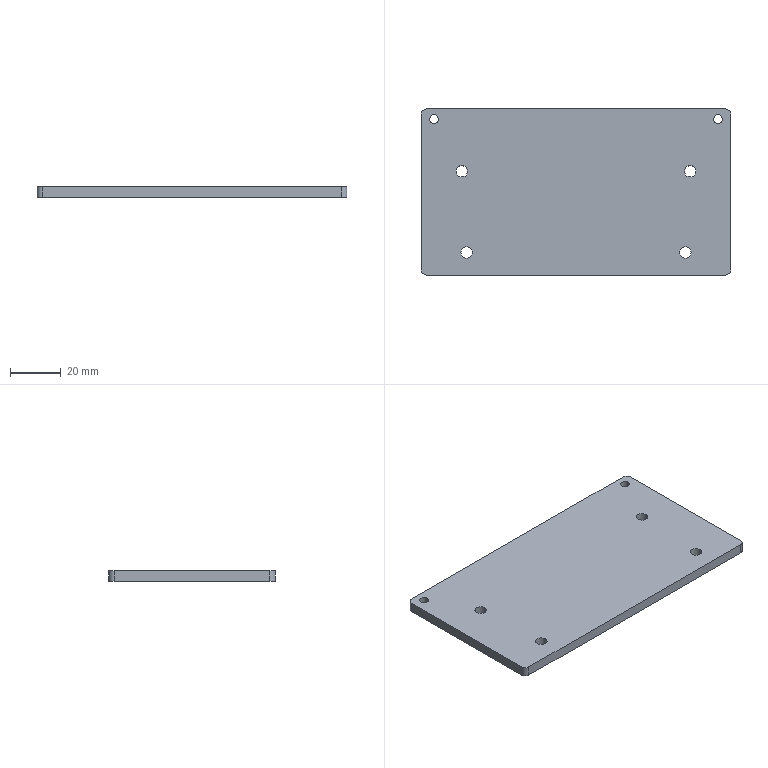Part | SolidWorks | features Extrusion 1, Fillet 1 | 1 solid | 22 faces | box 122 x 65.5 x 4 mm | volume 31619 mm3 | cylinder 16 | plane 6 | commonest cylinder face diameters 4.5 x8 3.5 x4 4 x4
STEP:
#1=CARTESIAN_POINT('',(40.9,-23.85,2.));
#2=VERTEX_POINT('',#1);
#3=CARTESIAN_POINT('',(45.4,-23.85,2.));
#4=VERTEX_POINT('',#3);
#5=CARTESIAN_POINT('',(43.15,-23.85,2.));
#6=DIRECTION('',(0.,0.,1.));
#7=DIRECTION('',(1.,0.,0.));
#8=AXIS2_PLACEMENT_3D('',#5,#6,#7);
#9=CIRCLE('',#8,2.25);
#10=EDGE_CURVE('',#2,#4,#9,.T.);
#11=ORIENTED_EDGE('',*,*,#10,.T.);
#12=CARTESIAN_POINT('',(45.4,-23.85,-2.));
#13=VERTEX_POINT('',#12);
#14=CARTESIAN_POINT('',(45.4,-23.85,2.));
#15=DIRECTION('',(0.,0.,-1.));
#16=VECTOR('',#15,1000.);
#17=LINE('',#14,#16);
#18=EDGE_CURVE('',#4,#13,#17,.T.);
#19=ORIENTED_EDGE('',*,*,#18,.T.);
#20=CARTESIAN_POINT('',(40.9,-23.85,-2.));
#21=VERTEX_POINT('',#20);
#22=CARTESIAN_POINT('',(43.15,-23.85,-2.));
#23=DIRECTION('',(0.,0.,1.));
#24=DIRECTION('',(1.,0.,0.));
#25=AXIS2_PLACEMENT_3D('',#22,#23,#24);
#26=CIRCLE('',#25,2.25);
#27=EDGE_CURVE('',#21,#13,#26,.T.);
#28=ORIENTED_EDGE('',*,*,#27,.F.);
#29=CARTESIAN_POINT('',(40.9,-23.85,2.));
#30=DIRECTION('',(0.,0.,-1.));
#31=VECTOR('',#30,1000.);
#32=LINE('',#29,#31);
#33=EDGE_CURVE('',#2,#21,#32,.T.);
#34=ORIENTED_EDGE('',*,*,#33,.F.);
#35=EDGE_LOOP('',(#11,#19,#28,#34));
#36=FACE_OUTER_BOUND('',#35,.T.);
#37=CARTESIAN_POINT('',(43.15,-23.85,2.));
#38=DIRECTION('',(0.,0.,-1.));
#39=DIRECTION('',(-1.,0.,0.));
#40=AXIS2_PLACEMENT_3D('',#37,#38,#39);
#41=CYLINDRICAL_SURFACE('',#40,2.25);
#42=ADVANCED_FACE('',(#36),#41,.F.);
#43=CARTESIAN_POINT('',(-45.4,-23.85,2.));
#44=VERTEX_POINT('',#43);
#45=CARTESIAN_POINT('',(-40.9,-23.85,2.));
#46=VERTEX_POINT('',#45);
#47=CARTESIAN_POINT('',(-43.15,-23.85,2.));
#48=DIRECTION('',(0.,0.,1.));
#49=DIRECTION('',(1.,0.,0.));
#50=AXIS2_PLACEMENT_3D('',#47,#48,#49);
#51=CIRCLE('',#50,2.25);
#52=EDGE_CURVE('',#44,#46,#51,.T.);
#53=ORIENTED_EDGE('',*,*,#52,.T.);
#54=CARTESIAN_POINT('',(-40.9,-23.85,-2.));
#55=VERTEX_POINT('',#54);
#56=CARTESIAN_POINT('',(-40.9,-23.85,2.));
#57=DIRECTION('',(0.,0.,-1.));
#58=VECTOR('',#57,1000.);
#59=LINE('',#56,#58);
#60=EDGE_CURVE('',#46,#55,#59,.T.);
#61=ORIENTED_EDGE('',*,*,#60,.T.);
#62=CARTESIAN_POINT('',(-45.4,-23.85,-2.));
#63=VERTEX_POINT('',#62);
#64=CARTESIAN_POINT('',(-43.15,-23.85,-2.));
#65=DIRECTION('',(0.,0.,1.));
#66=DIRECTION('',(1.,0.,0.));
#67=AXIS2_PLACEMENT_3D('',#64,#65,#66);
#68=CIRCLE('',#67,2.25);
#69=EDGE_CURVE('',#63,#55,#68,.T.);
#70=ORIENTED_EDGE('',*,*,#69,.F.);
#71=CARTESIAN_POINT('',(-45.4,-23.85,2.));
#72=DIRECTION('',(0.,0.,-1.));
#73=VECTOR('',#72,1000.);
#74=LINE('',#71,#73);
#75=EDGE_CURVE('',#44,#63,#74,.T.);
#76=ORIENTED_EDGE('',*,*,#75,.F.);
#77=EDGE_LOOP('',(#53,#61,#70,#76));
#78=FACE_OUTER_BOUND('',#77,.T.);
#79=CARTESIAN_POINT('',(-43.15,-23.85,2.));
#80=DIRECTION('',(0.,0.,-1.));
#81=DIRECTION('',(-1.,0.,0.));
#82=AXIS2_PLACEMENT_3D('',#79,#80,#81);
#83=CYLINDRICAL_SURFACE('',#82,2.25);
#84=ADVANCED_FACE('',(#78),#83,.F.);
#85=CARTESIAN_POINT('',(54.25,28.75,2.));
#86=VERTEX_POINT('',#85);
#87=CARTESIAN_POINT('',(57.75,28.75,2.));
#88=VERTEX_POINT('',#87);
#89=CARTESIAN_POINT('',(56.,28.75,2.));
#90=DIRECTION('',(0.,0.,1.));
#91=DIRECTION('',(-1.,0.,0.));
#92=AXIS2_PLACEMENT_3D('',#89,#90,#91);
#93=CIRCLE('',#92,1.75);
#94=EDGE_CURVE('',#86,#88,#93,.T.);
#95=ORIENTED_EDGE('',*,*,#94,.T.);
#96=CARTESIAN_POINT('',(57.75,28.75,-2.));
#97=VERTEX_POINT('',#96);
#98=CARTESIAN_POINT('',(57.75,28.75,2.));
#99=DIRECTION('',(0.,0.,-1.));
#100=VECTOR('',#99,1000.);
#101=LINE('',#98,#100);
#102=EDGE_CURVE('',#88,#97,#101,.T.);
#103=ORIENTED_EDGE('',*,*,#102,.T.);
#104=CARTESIAN_POINT('',(54.25,28.75,-2.));
#105=VERTEX_POINT('',#104);
#106=CARTESIAN_POINT('',(56.,28.75,-2.));
#107=DIRECTION('',(0.,0.,1.));
#108=DIRECTION('',(-1.,0.,0.));
#109=AXIS2_PLACEMENT_3D('',#106,#107,#108);
#110=CIRCLE('',#109,1.75);
#111=EDGE_CURVE('',#105,#97,#110,.T.);
#112=ORIENTED_EDGE('',*,*,#111,.F.);
#113=CARTESIAN_POINT('',(54.25,28.75,2.));
#114=DIRECTION('',(0.,0.,-1.));
#115=VECTOR('',#114,1000.);
#116=LINE('',#113,#115);
#117=EDGE_CURVE('',#86,#105,#116,.T.);
#118=ORIENTED_EDGE('',*,*,#117,.F.);
#119=EDGE_LOOP('',(#95,#103,#112,#118));
#120=FACE_OUTER_BOUND('',#119,.T.);
#121=CARTESIAN_POINT('',(56.,28.75,2.));
#122=DIRECTION('',(0.,0.,-1.));
#123=DIRECTION('',(-1.,0.,0.));
#124=AXIS2_PLACEMENT_3D('',#121,#122,#123);
#125=CYLINDRICAL_SURFACE('',#124,1.75);
#126=ADVANCED_FACE('',(#120),#125,.F.);
#127=CARTESIAN_POINT('',(42.75,8.15,2.));
#128=VERTEX_POINT('',#127);
#129=CARTESIAN_POINT('',(47.25,8.15,2.));
#130=VERTEX_POINT('',#129);
#131=CARTESIAN_POINT('',(45.,8.15,2.));
#132=DIRECTION('',(0.,0.,1.));
#133=DIRECTION('',(1.,0.,0.));
#134=AXIS2_PLACEMENT_3D('',#131,#132,#133);
#135=CIRCLE('',#134,2.25);
#136=EDGE_CURVE('',#128,#130,#135,.T.);
#137=ORIENTED_EDGE('',*,*,#136,.T.);
#138=CARTESIAN_POINT('',(47.25,8.15,-2.));
#139=VERTEX_POINT('',#138);
#140=CARTESIAN_POINT('',(47.25,8.15,2.));
#141=DIRECTION('',(0.,0.,-1.));
#142=VECTOR('',#141,1000.);
#143=LINE('',#140,#142);
#144=EDGE_CURVE('',#130,#139,#143,.T.);
#145=ORIENTED_EDGE('',*,*,#144,.T.);
#146=CARTESIAN_POINT('',(42.75,8.15,-2.));
#147=VERTEX_POINT('',#146);
#148=CARTESIAN_POINT('',(45.,8.15,-2.));
#149=DIRECTION('',(0.,0.,1.));
#150=DIRECTION('',(1.,0.,0.));
#151=AXIS2_PLACEMENT_3D('',#148,#149,#150);
#152=CIRCLE('',#151,2.25);
#153=EDGE_CURVE('',#147,#139,#152,.T.);
#154=ORIENTED_EDGE('',*,*,#153,.F.);
#155=CARTESIAN_POINT('',(42.75,8.15,2.));
#156=DIRECTION('',(0.,0.,-1.));
#157=VECTOR('',#156,1000.);
#158=LINE('',#155,#157);
#159=EDGE_CURVE('',#128,#147,#158,.T.);
#160=ORIENTED_EDGE('',*,*,#159,.F.);
#161=EDGE_LOOP('',(#137,#145,#154,#160));
#162=FACE_OUTER_BOUND('',#161,.T.);
#163=CARTESIAN_POINT('',(45.,8.15,2.));
#164=DIRECTION('',(0.,0.,-1.));
#165=DIRECTION('',(-1.,0.,0.));
#166=AXIS2_PLACEMENT_3D('',#163,#164,#165);
#167=CYLINDRICAL_SURFACE('',#166,2.25);
#168=ADVANCED_FACE('',(#162),#167,.F.);
#169=CARTESIAN_POINT('',(-47.25,8.15,2.));
#170=VERTEX_POINT('',#169);
#171=CARTESIAN_POINT('',(-42.75,8.15,2.));
#172=VERTEX_POINT('',#171);
#173=CARTESIAN_POINT('',(-45.,8.15,2.));
#174=DIRECTION('',(0.,0.,1.));
#175=DIRECTION('',(1.,0.,0.));
#176=AXIS2_PLACEMENT_3D('',#173,#174,#175);
#177=CIRCLE('',#176,2.25);
#178=EDGE_CURVE('',#170,#172,#177,.T.);
#179=ORIENTED_EDGE('',*,*,#178,.T.);
#180=CARTESIAN_POINT('',(-42.75,8.15,-2.));
#181=VERTEX_POINT('',#180);
#182=CARTESIAN_POINT('',(-42.75,8.15,2.));
#183=DIRECTION('',(0.,0.,-1.));
#184=VECTOR('',#183,1000.);
#185=LINE('',#182,#184);
#186=EDGE_CURVE('',#172,#181,#185,.T.);
#187=ORIENTED_EDGE('',*,*,#186,.T.);
#188=CARTESIAN_POINT('',(-47.25,8.15,-2.));
#189=VERTEX_POINT('',#188);
#190=CARTESIAN_POINT('',(-45.,8.15,-2.));
#191=DIRECTION('',(0.,0.,1.));
#192=DIRECTION('',(1.,0.,0.));
#193=AXIS2_PLACEMENT_3D('',#190,#191,#192);
#194=CIRCLE('',#193,2.25);
#195=EDGE_CURVE('',#189,#181,#194,.T.);
#196=ORIENTED_EDGE('',*,*,#195,.F.);
#197=CARTESIAN_POINT('',(-47.25,8.15,2.));
#198=DIRECTION('',(0.,0.,-1.));
#199=VECTOR('',#198,1000.);
#200=LINE('',#197,#199);
#201=EDGE_CURVE('',#170,#189,#200,.T.);
#202=ORIENTED_EDGE('',*,*,#201,.F.);
#203=EDGE_LOOP('',(#179,#187,#196,#202));
#204=FACE_OUTER_BOUND('',#203,.T.);
#205=CARTESIAN_POINT('',(-45.,8.15,2.));
#206=DIRECTION('',(0.,0.,-1.));
#207=DIRECTION('',(-1.,0.,0.));
#208=AXIS2_PLACEMENT_3D('',#205,#206,#207);
#209=CYLINDRICAL_SURFACE('',#208,2.25);
#210=ADVANCED_FACE('',(#204),#209,.F.);
#211=CARTESIAN_POINT('',(-57.75,28.75,2.));
#212=VERTEX_POINT('',#211);
#213=CARTESIAN_POINT('',(-54.25,28.75,2.));
#214=VERTEX_POINT('',#213);
#215=CARTESIAN_POINT('',(-56.,28.75,2.));
#216=DIRECTION('',(0.,0.,1.));
#217=DIRECTION('',(1.,0.,0.));
#218=AXIS2_PLACEMENT_3D('',#215,#216,#217);
#219=CIRCLE('',#218,1.75);
#220=EDGE_CURVE('',#212,#214,#219,.T.);
#221=ORIENTED_EDGE('',*,*,#220,.T.);
#222=CARTESIAN_POINT('',(-54.25,28.75,-2.));
#223=VERTEX_POINT('',#222);
#224=CARTESIAN_POINT('',(-54.25,28.75,2.));
#225=DIRECTION('',(0.,0.,-1.));
#226=VECTOR('',#225,1000.);
#227=LINE('',#224,#226);
#228=EDGE_CURVE('',#214,#223,#227,.T.);
#229=ORIENTED_EDGE('',*,*,#228,.T.);
#230=CARTESIAN_POINT('',(-57.75,28.75,-2.));
#231=VERTEX_POINT('',#230);
#232=CARTESIAN_POINT('',(-56.,28.75,-2.));
#233=DIRECTION('',(0.,0.,1.));
#234=DIRECTION('',(1.,0.,0.));
#235=AXIS2_PLACEMENT_3D('',#232,#233,#234);
#236=CIRCLE('',#235,1.75);
#237=EDGE_CURVE('',#231,#223,#236,.T.);
#238=ORIENTED_EDGE('',*,*,#237,.F.);
#239=CARTESIAN_POINT('',(-57.75,28.75,2.));
#240=DIRECTION('',(0.,0.,-1.));
#241=VECTOR('',#240,1000.);
#242=LINE('',#239,#241);
#243=EDGE_CURVE('',#212,#231,#242,.T.);
#244=ORIENTED_EDGE('',*,*,#243,.F.);
#245=EDGE_LOOP('',(#221,#229,#238,#244));
#246=FACE_OUTER_BOUND('',#245,.T.);
#247=CARTESIAN_POINT('',(-56.,28.75,2.));
#248=DIRECTION('',(0.,0.,-1.));
#249=DIRECTION('',(-1.,0.,0.));
#250=AXIS2_PLACEMENT_3D('',#247,#248,#249);
#251=CYLINDRICAL_SURFACE('',#250,1.75);
#252=ADVANCED_FACE('',(#246),#251,.F.);
#253=ORIENTED_EDGE('',*,*,#52,.F.);
#254=CARTESIAN_POINT('',(-43.15,-23.85,2.));
#255=DIRECTION('',(0.,0.,1.));
#256=DIRECTION('',(1.,0.,0.));
#257=AXIS2_PLACEMENT_3D('',#254,#255,#256);
#258=CIRCLE('',#257,2.25);
#259=EDGE_CURVE('',#46,#44,#258,.T.);
#260=ORIENTED_EDGE('',*,*,#259,.F.);
#261=EDGE_LOOP('',(#253,#260));
#262=FACE_BOUND('',#261,.T.);
#263=ORIENTED_EDGE('',*,*,#136,.F.);
#264=CARTESIAN_POINT('',(45.,8.15,2.));
#265=DIRECTION('',(0.,0.,1.));
#266=DIRECTION('',(1.,0.,0.));
#267=AXIS2_PLACEMENT_3D('',#264,#265,#266);
#268=CIRCLE('',#267,2.25);
#269=EDGE_CURVE('',#130,#128,#268,.T.);
#270=ORIENTED_EDGE('',*,*,#269,.F.);
#271=EDGE_LOOP('',(#263,#270));
#272=FACE_BOUND('',#271,.T.);
#273=ORIENTED_EDGE('',*,*,#220,.F.);
#274=CARTESIAN_POINT('',(-56.,28.75,2.));
#275=DIRECTION('',(0.,0.,1.));
#276=DIRECTION('',(1.,0.,0.));
#277=AXIS2_PLACEMENT_3D('',#274,#275,#276);
#278=CIRCLE('',#277,1.75);
#279=EDGE_CURVE('',#214,#212,#278,.T.);
#280=ORIENTED_EDGE('',*,*,#279,.F.);
#281=EDGE_LOOP('',(#273,#280));
#282=FACE_BOUND('',#281,.T.);
#283=CARTESIAN_POINT('',(-59.,-32.75,2.));
#284=VERTEX_POINT('',#283);
#285=CARTESIAN_POINT('',(59.,-32.75,2.));
#286=VERTEX_POINT('',#285);
#287=CARTESIAN_POINT('',(-61.,-32.75,2.));
#288=DIRECTION('',(1.,0.,0.));
#289=VECTOR('',#288,1000.);
#290=LINE('',#287,#289);
#291=EDGE_CURVE('',#284,#286,#290,.T.);
#292=ORIENTED_EDGE('',*,*,#291,.T.);
#293=CARTESIAN_POINT('',(61.,-30.75,2.));
#294=VERTEX_POINT('',#293);
#295=CARTESIAN_POINT('',(59.,-30.75,2.));
#296=DIRECTION('',(0.,0.,1.));
#297=DIRECTION('',(1.,0.,0.));
#298=AXIS2_PLACEMENT_3D('',#295,#296,#297);
#299=CIRCLE('',#298,2.);
#300=EDGE_CURVE('',#286,#294,#299,.T.);
#301=ORIENTED_EDGE('',*,*,#300,.T.);
#302=CARTESIAN_POINT('',(61.,30.75,2.));
#303=VERTEX_POINT('',#302);
#304=CARTESIAN_POINT('',(61.,32.75,2.));
#305=DIRECTION('',(0.,1.,0.));
#306=VECTOR('',#305,1000.);
#307=LINE('',#304,#306);
#308=EDGE_CURVE('',#294,#303,#307,.T.);
#309=ORIENTED_EDGE('',*,*,#308,.T.);
#310=CARTESIAN_POINT('',(59.,32.75,2.));
#311=VERTEX_POINT('',#310);
#312=CARTESIAN_POINT('',(59.,30.75,2.));
#313=DIRECTION('',(0.,0.,1.));
#314=DIRECTION('',(1.,0.,0.));
#315=AXIS2_PLACEMENT_3D('',#312,#313,#314);
#316=CIRCLE('',#315,2.);
#317=EDGE_CURVE('',#303,#311,#316,.T.);
#318=ORIENTED_EDGE('',*,*,#317,.T.);
#319=CARTESIAN_POINT('',(-59.,32.75,2.));
#320=VERTEX_POINT('',#319);
#321=CARTESIAN_POINT('',(-61.,32.75,2.));
#322=DIRECTION('',(-1.,0.,0.));
#323=VECTOR('',#322,1000.);
#324=LINE('',#321,#323);
#325=EDGE_CURVE('',#311,#320,#324,.T.);
#326=ORIENTED_EDGE('',*,*,#325,.T.);
#327=CARTESIAN_POINT('',(-61.,30.75,2.));
#328=VERTEX_POINT('',#327);
#329=CARTESIAN_POINT('',(-59.,30.75,2.));
#330=DIRECTION('',(0.,0.,1.));
#331=DIRECTION('',(1.,0.,0.));
#332=AXIS2_PLACEMENT_3D('',#329,#330,#331);
#333=CIRCLE('',#332,2.);
#334=EDGE_CURVE('',#320,#328,#333,.T.);
#335=ORIENTED_EDGE('',*,*,#334,.T.);
#336=CARTESIAN_POINT('',(-61.,-30.75,2.));
#337=VERTEX_POINT('',#336);
#338=CARTESIAN_POINT('',(-61.,32.75,2.));
#339=DIRECTION('',(0.,-1.,0.));
#340=VECTOR('',#339,1000.);
#341=LINE('',#338,#340);
#342=EDGE_CURVE('',#328,#337,#341,.T.);
#343=ORIENTED_EDGE('',*,*,#342,.T.);
#344=CARTESIAN_POINT('',(-59.,-30.75,2.));
#345=DIRECTION('',(0.,0.,1.));
#346=DIRECTION('',(1.,0.,0.));
#347=AXIS2_PLACEMENT_3D('',#344,#345,#346);
#348=CIRCLE('',#347,2.);
#349=EDGE_CURVE('',#337,#284,#348,.T.);
#350=ORIENTED_EDGE('',*,*,#349,.T.);
#351=EDGE_LOOP('',(#292,#301,#309,#318,#326,#335,#343,#350));
#352=FACE_OUTER_BOUND('',#351,.T.);
#353=ORIENTED_EDGE('',*,*,#178,.F.);
#354=CARTESIAN_POINT('',(-45.,8.15,2.));
#355=DIRECTION('',(0.,0.,1.));
#356=DIRECTION('',(1.,0.,0.));
#357=AXIS2_PLACEMENT_3D('',#354,#355,#356);
#358=CIRCLE('',#357,2.25);
#359=EDGE_CURVE('',#172,#170,#358,.T.);
#360=ORIENTED_EDGE('',*,*,#359,.F.);
#361=EDGE_LOOP('',(#353,#360));
#362=FACE_BOUND('',#361,.T.);
#363=ORIENTED_EDGE('',*,*,#94,.F.);
#364=CARTESIAN_POINT('',(56.,28.75,2.));
#365=DIRECTION('',(0.,0.,1.));
#366=DIRECTION('',(-1.,0.,0.));
#367=AXIS2_PLACEMENT_3D('',#364,#365,#366);
#368=CIRCLE('',#367,1.75);
#369=EDGE_CURVE('',#88,#86,#368,.T.);
#370=ORIENTED_EDGE('',*,*,#369,.F.);
#371=EDGE_LOOP('',(#363,#370));
#372=FACE_BOUND('',#371,.T.);
#373=ORIENTED_EDGE('',*,*,#10,.F.);
#374=CARTESIAN_POINT('',(43.15,-23.85,2.));
#375=DIRECTION('',(0.,0.,1.));
#376=DIRECTION('',(1.,0.,0.));
#377=AXIS2_PLACEMENT_3D('',#374,#375,#376);
#378=CIRCLE('',#377,2.25);
#379=EDGE_CURVE('',#4,#2,#378,.T.);
#380=ORIENTED_EDGE('',*,*,#379,.F.);
#381=EDGE_LOOP('',(#373,#380));
#382=FACE_BOUND('',#381,.T.);
#383=CARTESIAN_POINT('',(0.,0.,2.));
#384=DIRECTION('',(0.,0.,1.));
#385=DIRECTION('',(1.,0.,0.));
#386=AXIS2_PLACEMENT_3D('',#383,#384,#385);
#387=PLANE('',#386);
#388=ADVANCED_FACE('',(#262,#272,#282,#352,#362,#372,#382),#387,.T.);
#389=CARTESIAN_POINT('',(61.,-30.75,-2.));
#390=VERTEX_POINT('',#389);
#391=CARTESIAN_POINT('',(61.,30.75,-2.));
#392=VERTEX_POINT('',#391);
#393=CARTESIAN_POINT('',(61.,32.75,-2.));
#394=DIRECTION('',(0.,1.,0.));
#395=VECTOR('',#394,1000.);
#396=LINE('',#393,#395);
#397=EDGE_CURVE('',#390,#392,#396,.T.);
#398=ORIENTED_EDGE('',*,*,#397,.F.);
#399=CARTESIAN_POINT('',(59.,-32.75,-2.));
#400=VERTEX_POINT('',#399);
#401=CARTESIAN_POINT('',(59.,-30.75,-2.));
#402=DIRECTION('',(0.,0.,-1.));
#403=DIRECTION('',(1.,0.,0.));
#404=AXIS2_PLACEMENT_3D('',#401,#402,#403);
#405=CIRCLE('',#404,2.);
#406=EDGE_CURVE('',#390,#400,#405,.T.);
#407=ORIENTED_EDGE('',*,*,#406,.T.);
#408=CARTESIAN_POINT('',(-59.,-32.75,-2.));
#409=VERTEX_POINT('',#408);
#410=CARTESIAN_POINT('',(-61.,-32.75,-2.));
#411=DIRECTION('',(1.,0.,0.));
#412=VECTOR('',#411,1000.);
#413=LINE('',#410,#412);
#414=EDGE_CURVE('',#409,#400,#413,.T.);
#415=ORIENTED_EDGE('',*,*,#414,.F.);
#416=CARTESIAN_POINT('',(-61.,-30.75,-2.));
#417=VERTEX_POINT('',#416);
#418=CARTESIAN_POINT('',(-59.,-30.75,-2.));
#419=DIRECTION('',(0.,0.,-1.));
#420=DIRECTION('',(1.,0.,0.));
#421=AXIS2_PLACEMENT_3D('',#418,#419,#420);
#422=CIRCLE('',#421,2.);
#423=EDGE_CURVE('',#409,#417,#422,.T.);
#424=ORIENTED_EDGE('',*,*,#423,.T.);
#425=CARTESIAN_POINT('',(-61.,30.75,-2.));
#426=VERTEX_POINT('',#425);
#427=CARTESIAN_POINT('',(-61.,32.75,-2.));
#428=DIRECTION('',(0.,-1.,0.));
#429=VECTOR('',#428,1000.);
#430=LINE('',#427,#429);
#431=EDGE_CURVE('',#426,#417,#430,.T.);
#432=ORIENTED_EDGE('',*,*,#431,.F.);
#433=CARTESIAN_POINT('',(-59.,32.75,-2.));
#434=VERTEX_POINT('',#433);
#435=CARTESIAN_POINT('',(-59.,30.75,-2.));
#436=DIRECTION('',(0.,0.,-1.));
#437=DIRECTION('',(1.,0.,0.));
#438=AXIS2_PLACEMENT_3D('',#435,#436,#437);
#439=CIRCLE('',#438,2.);
#440=EDGE_CURVE('',#426,#434,#439,.T.);
#441=ORIENTED_EDGE('',*,*,#440,.T.);
#442=CARTESIAN_POINT('',(59.,32.75,-2.));
#443=VERTEX_POINT('',#442);
#444=CARTESIAN_POINT('',(-61.,32.75,-2.));
#445=DIRECTION('',(-1.,0.,0.));
#446=VECTOR('',#445,1000.);
#447=LINE('',#444,#446);
#448=EDGE_CURVE('',#443,#434,#447,.T.);
#449=ORIENTED_EDGE('',*,*,#448,.F.);
#450=CARTESIAN_POINT('',(59.,30.75,-2.));
#451=DIRECTION('',(0.,0.,-1.));
#452=DIRECTION('',(1.,0.,0.));
#453=AXIS2_PLACEMENT_3D('',#450,#451,#452);
#454=CIRCLE('',#453,2.);
#455=EDGE_CURVE('',#443,#392,#454,.T.);
#456=ORIENTED_EDGE('',*,*,#455,.T.);
#457=EDGE_LOOP('',(#398,#407,#415,#424,#432,#441,#449,#456));
#458=FACE_OUTER_BOUND('',#457,.T.);
#459=ORIENTED_EDGE('',*,*,#237,.T.);
#460=CARTESIAN_POINT('',(-56.,28.75,-2.));
#461=DIRECTION('',(0.,0.,1.));
#462=DIRECTION('',(1.,0.,0.));
#463=AXIS2_PLACEMENT_3D('',#460,#461,#462);
#464=CIRCLE('',#463,1.75);
#465=EDGE_CURVE('',#223,#231,#464,.T.);
#466=ORIENTED_EDGE('',*,*,#465,.T.);
#467=EDGE_LOOP('',(#459,#466));
#468=FACE_BOUND('',#467,.T.);
#469=ORIENTED_EDGE('',*,*,#195,.T.);
#470=CARTESIAN_POINT('',(-45.,8.15,-2.));
#471=DIRECTION('',(0.,0.,1.));
#472=DIRECTION('',(1.,0.,0.));
#473=AXIS2_PLACEMENT_3D('',#470,#471,#472);
#474=CIRCLE('',#473,2.25);
#475=EDGE_CURVE('',#181,#189,#474,.T.);
#476=ORIENTED_EDGE('',*,*,#475,.T.);
#477=EDGE_LOOP('',(#469,#476));
#478=FACE_BOUND('',#477,.T.);
#479=ORIENTED_EDGE('',*,*,#153,.T.);
#480=CARTESIAN_POINT('',(45.,8.15,-2.));
#481=DIRECTION('',(0.,0.,1.));
#482=DIRECTION('',(1.,0.,0.));
#483=AXIS2_PLACEMENT_3D('',#480,#481,#482);
#484=CIRCLE('',#483,2.25);
#485=EDGE_CURVE('',#139,#147,#484,.T.);
#486=ORIENTED_EDGE('',*,*,#485,.T.);
#487=EDGE_LOOP('',(#479,#486));
#488=FACE_BOUND('',#487,.T.);
#489=ORIENTED_EDGE('',*,*,#111,.T.);
#490=CARTESIAN_POINT('',(56.,28.75,-2.));
#491=DIRECTION('',(0.,0.,1.));
#492=DIRECTION('',(-1.,0.,0.));
#493=AXIS2_PLACEMENT_3D('',#490,#491,#492);
#494=CIRCLE('',#493,1.75);
#495=EDGE_CURVE('',#97,#105,#494,.T.);
#496=ORIENTED_EDGE('',*,*,#495,.T.);
#497=EDGE_LOOP('',(#489,#496));
#498=FACE_BOUND('',#497,.T.);
#499=ORIENTED_EDGE('',*,*,#69,.T.);
#500=CARTESIAN_POINT('',(-43.15,-23.85,-2.));
#501=DIRECTION('',(0.,0.,1.));
#502=DIRECTION('',(1.,0.,0.));
#503=AXIS2_PLACEMENT_3D('',#500,#501,#502);
#504=CIRCLE('',#503,2.25);
#505=EDGE_CURVE('',#55,#63,#504,.T.);
#506=ORIENTED_EDGE('',*,*,#505,.T.);
#507=EDGE_LOOP('',(#499,#506));
#508=FACE_BOUND('',#507,.T.);
#509=ORIENTED_EDGE('',*,*,#27,.T.);
#510=CARTESIAN_POINT('',(43.15,-23.85,-2.));
#511=DIRECTION('',(0.,0.,1.));
#512=DIRECTION('',(1.,0.,0.));
#513=AXIS2_PLACEMENT_3D('',#510,#511,#512);
#514=CIRCLE('',#513,2.25);
#515=EDGE_CURVE('',#13,#21,#514,.T.);
#516=ORIENTED_EDGE('',*,*,#515,.T.);
#517=EDGE_LOOP('',(#509,#516));
#518=FACE_BOUND('',#517,.T.);
#519=CARTESIAN_POINT('',(0.,0.,-2.));
#520=DIRECTION('',(0.,0.,1.));
#521=DIRECTION('',(1.,0.,0.));
#522=AXIS2_PLACEMENT_3D('',#519,#520,#521);
#523=PLANE('',#522);
#524=ADVANCED_FACE('',(#458,#468,#478,#488,#498,#508,#518),#523,.F.);
#525=ORIENTED_EDGE('',*,*,#308,.F.);
#526=CARTESIAN_POINT('',(61.,-30.75,2.));
#527=DIRECTION('',(0.,0.,-1.));
#528=VECTOR('',#527,1000.);
#529=LINE('',#526,#528);
#530=EDGE_CURVE('',#294,#390,#529,.T.);
#531=ORIENTED_EDGE('',*,*,#530,.T.);
#532=ORIENTED_EDGE('',*,*,#397,.T.);
#533=CARTESIAN_POINT('',(61.,30.75,2.));
#534=DIRECTION('',(0.,0.,1.));
#535=VECTOR('',#534,1000.);
#536=LINE('',#533,#535);
#537=EDGE_CURVE('',#392,#303,#536,.T.);
#538=ORIENTED_EDGE('',*,*,#537,.T.);
#539=EDGE_LOOP('',(#525,#531,#532,#538));
#540=FACE_OUTER_BOUND('',#539,.T.);
#541=CARTESIAN_POINT('',(61.,32.75,2.));
#542=DIRECTION('',(-1.,0.,0.));
#543=DIRECTION('',(0.,-1.,0.));
#544=AXIS2_PLACEMENT_3D('',#541,#542,#543);
#545=PLANE('',#544);
#546=ADVANCED_FACE('',(#540),#545,.F.);
#547=ORIENTED_EDGE('',*,*,#325,.F.);
#548=CARTESIAN_POINT('',(59.,32.75,2.));
#549=DIRECTION('',(0.,0.,-1.));
#550=VECTOR('',#549,1000.);
#551=LINE('',#548,#550);
#552=EDGE_CURVE('',#311,#443,#551,.T.);
#553=ORIENTED_EDGE('',*,*,#552,.T.);
#554=ORIENTED_EDGE('',*,*,#448,.T.);
#555=CARTESIAN_POINT('',(-59.,32.75,2.));
#556=DIRECTION('',(0.,0.,1.));
#557=VECTOR('',#556,1000.);
#558=LINE('',#555,#557);
#559=EDGE_CURVE('',#434,#320,#558,.T.);
#560=ORIENTED_EDGE('',*,*,#559,.T.);
#561=EDGE_LOOP('',(#547,#553,#554,#560));
#562=FACE_OUTER_BOUND('',#561,.T.);
#563=CARTESIAN_POINT('',(-61.,32.75,2.));
#564=DIRECTION('',(0.,-1.,0.));
#565=DIRECTION('',(1.,0.,0.));
#566=AXIS2_PLACEMENT_3D('',#563,#564,#565);
#567=PLANE('',#566);
#568=ADVANCED_FACE('',(#562),#567,.F.);
#569=ORIENTED_EDGE('',*,*,#431,.T.);
#570=CARTESIAN_POINT('',(-61.,-30.75,2.));
#571=DIRECTION('',(0.,0.,1.));
#572=VECTOR('',#571,1000.);
#573=LINE('',#570,#572);
#574=EDGE_CURVE('',#417,#337,#573,.T.);
#575=ORIENTED_EDGE('',*,*,#574,.T.);
#576=ORIENTED_EDGE('',*,*,#342,.F.);
#577=CARTESIAN_POINT('',(-61.,30.75,2.));
#578=DIRECTION('',(0.,0.,-1.));
#579=VECTOR('',#578,1000.);
#580=LINE('',#577,#579);
#581=EDGE_CURVE('',#328,#426,#580,.T.);
#582=ORIENTED_EDGE('',*,*,#581,.T.);
#583=EDGE_LOOP('',(#569,#575,#576,#582));
#584=FACE_OUTER_BOUND('',#583,.T.);
#585=CARTESIAN_POINT('',(-61.,32.75,2.));
#586=DIRECTION('',(1.,0.,0.));
#587=DIRECTION('',(0.,1.,0.));
#588=AXIS2_PLACEMENT_3D('',#585,#586,#587);
#589=PLANE('',#588);
#590=ADVANCED_FACE('',(#584),#589,.F.);
#591=ORIENTED_EDGE('',*,*,#414,.T.);
#592=CARTESIAN_POINT('',(59.,-32.75,2.));
#593=DIRECTION('',(0.,0.,1.));
#594=VECTOR('',#593,1000.);
#595=LINE('',#592,#594);
#596=EDGE_CURVE('',#400,#286,#595,.T.);
#597=ORIENTED_EDGE('',*,*,#596,.T.);
#598=ORIENTED_EDGE('',*,*,#291,.F.);
#599=CARTESIAN_POINT('',(-59.,-32.75,2.));
#600=DIRECTION('',(0.,0.,-1.));
#601=VECTOR('',#600,1000.);
#602=LINE('',#599,#601);
#603=EDGE_CURVE('',#284,#409,#602,.T.);
#604=ORIENTED_EDGE('',*,*,#603,.T.);
#605=EDGE_LOOP('',(#591,#597,#598,#604));
#606=FACE_OUTER_BOUND('',#605,.T.);
#607=CARTESIAN_POINT('',(-61.,-32.75,2.));
#608=DIRECTION('',(0.,1.,0.));
#609=DIRECTION('',(0.,0.,1.));
#610=AXIS2_PLACEMENT_3D('',#607,#608,#609);
#611=PLANE('',#610);
#612=ADVANCED_FACE('',(#606),#611,.F.);
#613=ORIENTED_EDGE('',*,*,#228,.F.);
#614=ORIENTED_EDGE('',*,*,#279,.T.);
#615=ORIENTED_EDGE('',*,*,#243,.T.);
#616=ORIENTED_EDGE('',*,*,#465,.F.);
#617=EDGE_LOOP('',(#613,#614,#615,#616));
#618=FACE_OUTER_BOUND('',#617,.T.);
#619=CARTESIAN_POINT('',(-56.,28.75,2.));
#620=DIRECTION('',(0.,0.,-1.));
#621=DIRECTION('',(-1.,0.,0.));
#622=AXIS2_PLACEMENT_3D('',#619,#620,#621);
#623=CYLINDRICAL_SURFACE('',#622,1.75);
#624=ADVANCED_FACE('',(#618),#623,.F.);
#625=ORIENTED_EDGE('',*,*,#186,.F.);
#626=ORIENTED_EDGE('',*,*,#359,.T.);
#627=ORIENTED_EDGE('',*,*,#201,.T.);
#628=ORIENTED_EDGE('',*,*,#475,.F.);
#629=EDGE_LOOP('',(#625,#626,#627,#628));
#630=FACE_OUTER_BOUND('',#629,.T.);
#631=CARTESIAN_POINT('',(-45.,8.15,2.));
#632=DIRECTION('',(0.,0.,-1.));
#633=DIRECTION('',(-1.,0.,0.));
#634=AXIS2_PLACEMENT_3D('',#631,#632,#633);
#635=CYLINDRICAL_SURFACE('',#634,2.25);
#636=ADVANCED_FACE('',(#630),#635,.F.);
#637=ORIENTED_EDGE('',*,*,#144,.F.);
#638=ORIENTED_EDGE('',*,*,#269,.T.);
#639=ORIENTED_EDGE('',*,*,#159,.T.);
#640=ORIENTED_EDGE('',*,*,#485,.F.);
#641=EDGE_LOOP('',(#637,#638,#639,#640));
#642=FACE_OUTER_BOUND('',#641,.T.);
#643=CARTESIAN_POINT('',(45.,8.15,2.));
#644=DIRECTION('',(0.,0.,-1.));
#645=DIRECTION('',(-1.,0.,0.));
#646=AXIS2_PLACEMENT_3D('',#643,#644,#645);
#647=CYLINDRICAL_SURFACE('',#646,2.25);
#648=ADVANCED_FACE('',(#642),#647,.F.);
#649=ORIENTED_EDGE('',*,*,#102,.F.);
#650=ORIENTED_EDGE('',*,*,#369,.T.);
#651=ORIENTED_EDGE('',*,*,#117,.T.);
#652=ORIENTED_EDGE('',*,*,#495,.F.);
#653=EDGE_LOOP('',(#649,#650,#651,#652));
#654=FACE_OUTER_BOUND('',#653,.T.);
#655=CARTESIAN_POINT('',(56.,28.75,2.));
#656=DIRECTION('',(0.,0.,-1.));
#657=DIRECTION('',(-1.,0.,0.));
#658=AXIS2_PLACEMENT_3D('',#655,#656,#657);
#659=CYLINDRICAL_SURFACE('',#658,1.75);
#660=ADVANCED_FACE('',(#654),#659,.F.);
#661=ORIENTED_EDGE('',*,*,#60,.F.);
#662=ORIENTED_EDGE('',*,*,#259,.T.);
#663=ORIENTED_EDGE('',*,*,#75,.T.);
#664=ORIENTED_EDGE('',*,*,#505,.F.);
#665=EDGE_LOOP('',(#661,#662,#663,#664));
#666=FACE_OUTER_BOUND('',#665,.T.);
#667=CARTESIAN_POINT('',(-43.15,-23.85,2.));
#668=DIRECTION('',(0.,0.,-1.));
#669=DIRECTION('',(-1.,0.,0.));
#670=AXIS2_PLACEMENT_3D('',#667,#668,#669);
#671=CYLINDRICAL_SURFACE('',#670,2.25);
#672=ADVANCED_FACE('',(#666),#671,.F.);
#673=ORIENTED_EDGE('',*,*,#18,.F.);
#674=ORIENTED_EDGE('',*,*,#379,.T.);
#675=ORIENTED_EDGE('',*,*,#33,.T.);
#676=ORIENTED_EDGE('',*,*,#515,.F.);
#677=EDGE_LOOP('',(#673,#674,#675,#676));
#678=FACE_OUTER_BOUND('',#677,.T.);
#679=CARTESIAN_POINT('',(43.15,-23.85,2.));
#680=DIRECTION('',(0.,0.,-1.));
#681=DIRECTION('',(-1.,0.,0.));
#682=AXIS2_PLACEMENT_3D('',#679,#680,#681);
#683=CYLINDRICAL_SURFACE('',#682,2.25);
#684=ADVANCED_FACE('',(#678),#683,.F.);
#685=ORIENTED_EDGE('',*,*,#300,.F.);
#686=ORIENTED_EDGE('',*,*,#596,.F.);
#687=ORIENTED_EDGE('',*,*,#406,.F.);
#688=ORIENTED_EDGE('',*,*,#530,.F.);
#689=EDGE_LOOP('',(#685,#686,#687,#688));
#690=FACE_OUTER_BOUND('',#689,.T.);
#691=CARTESIAN_POINT('',(59.,-30.75,2.));
#692=DIRECTION('',(0.,0.,-1.));
#693=DIRECTION('',(-1.,0.,0.));
#694=AXIS2_PLACEMENT_3D('',#691,#692,#693);
#695=CYLINDRICAL_SURFACE('',#694,2.);
#696=ADVANCED_FACE('',(#690),#695,.T.);
#697=ORIENTED_EDGE('',*,*,#317,.F.);
#698=ORIENTED_EDGE('',*,*,#537,.F.);
#699=ORIENTED_EDGE('',*,*,#455,.F.);
#700=ORIENTED_EDGE('',*,*,#552,.F.);
#701=EDGE_LOOP('',(#697,#698,#699,#700));
#702=FACE_OUTER_BOUND('',#701,.T.);
#703=CARTESIAN_POINT('',(59.,30.75,2.));
#704=DIRECTION('',(0.,0.,-1.));
#705=DIRECTION('',(-1.,0.,0.));
#706=AXIS2_PLACEMENT_3D('',#703,#704,#705);
#707=CYLINDRICAL_SURFACE('',#706,2.);
#708=ADVANCED_FACE('',(#702),#707,.T.);
#709=ORIENTED_EDGE('',*,*,#349,.F.);
#710=ORIENTED_EDGE('',*,*,#574,.F.);
#711=ORIENTED_EDGE('',*,*,#423,.F.);
#712=ORIENTED_EDGE('',*,*,#603,.F.);
#713=EDGE_LOOP('',(#709,#710,#711,#712));
#714=FACE_OUTER_BOUND('',#713,.T.);
#715=CARTESIAN_POINT('',(-59.,-30.75,2.));
#716=DIRECTION('',(0.,0.,-1.));
#717=DIRECTION('',(-1.,0.,0.));
#718=AXIS2_PLACEMENT_3D('',#715,#716,#717);
#719=CYLINDRICAL_SURFACE('',#718,2.);
#720=ADVANCED_FACE('',(#714),#719,.T.);
#721=ORIENTED_EDGE('',*,*,#334,.F.);
#722=ORIENTED_EDGE('',*,*,#559,.F.);
#723=ORIENTED_EDGE('',*,*,#440,.F.);
#724=ORIENTED_EDGE('',*,*,#581,.F.);
#725=EDGE_LOOP('',(#721,#722,#723,#724));
#726=FACE_OUTER_BOUND('',#725,.T.);
#727=CARTESIAN_POINT('',(-59.,30.75,2.));
#728=DIRECTION('',(0.,0.,-1.));
#729=DIRECTION('',(-1.,0.,0.));
#730=AXIS2_PLACEMENT_3D('',#727,#728,#729);
#731=CYLINDRICAL_SURFACE('',#730,2.);
#732=ADVANCED_FACE('',(#726),#731,.T.);
#733=CLOSED_SHELL('',(#42,#84,#126,#168,#210,#252,#388,#524,#546,#568,#590,#612,#624,#636,#648,#660,#672,#684,#696,#708,#720,#732));
#734=MANIFOLD_SOLID_BREP('',#733);
#735=CARTESIAN_POINT('',(0.,0.,0.));
#736=DIRECTION('',(0.,0.,1.));
#737=DIRECTION('',(1.,0.,0.));
#738=AXIS2_PLACEMENT_3D('',#735,#736,#737);
#739=(LENGTH_UNIT()NAMED_UNIT(*)SI_UNIT(.MILLI.,.METRE.));
#740=UNCERTAINTY_MEASURE_WITH_UNIT(LENGTH_MEASURE(0.00001),#739,'','');
#741=(NAMED_UNIT(*)PLANE_ANGLE_UNIT()SI_UNIT($,.RADIAN.));
#742=(NAMED_UNIT(*)SI_UNIT($,.STERADIAN.)SOLID_ANGLE_UNIT());
#743=(GEOMETRIC_REPRESENTATION_CONTEXT(3)GLOBAL_UNCERTAINTY_ASSIGNED_CONTEXT((#740))GLOBAL_UNIT_ASSIGNED_CONTEXT((#739,#741,#742))REPRESENTATION_CONTEXT('',''));
#744=ADVANCED_BREP_SHAPE_REPRESENTATION('',(#734,#738),#743);